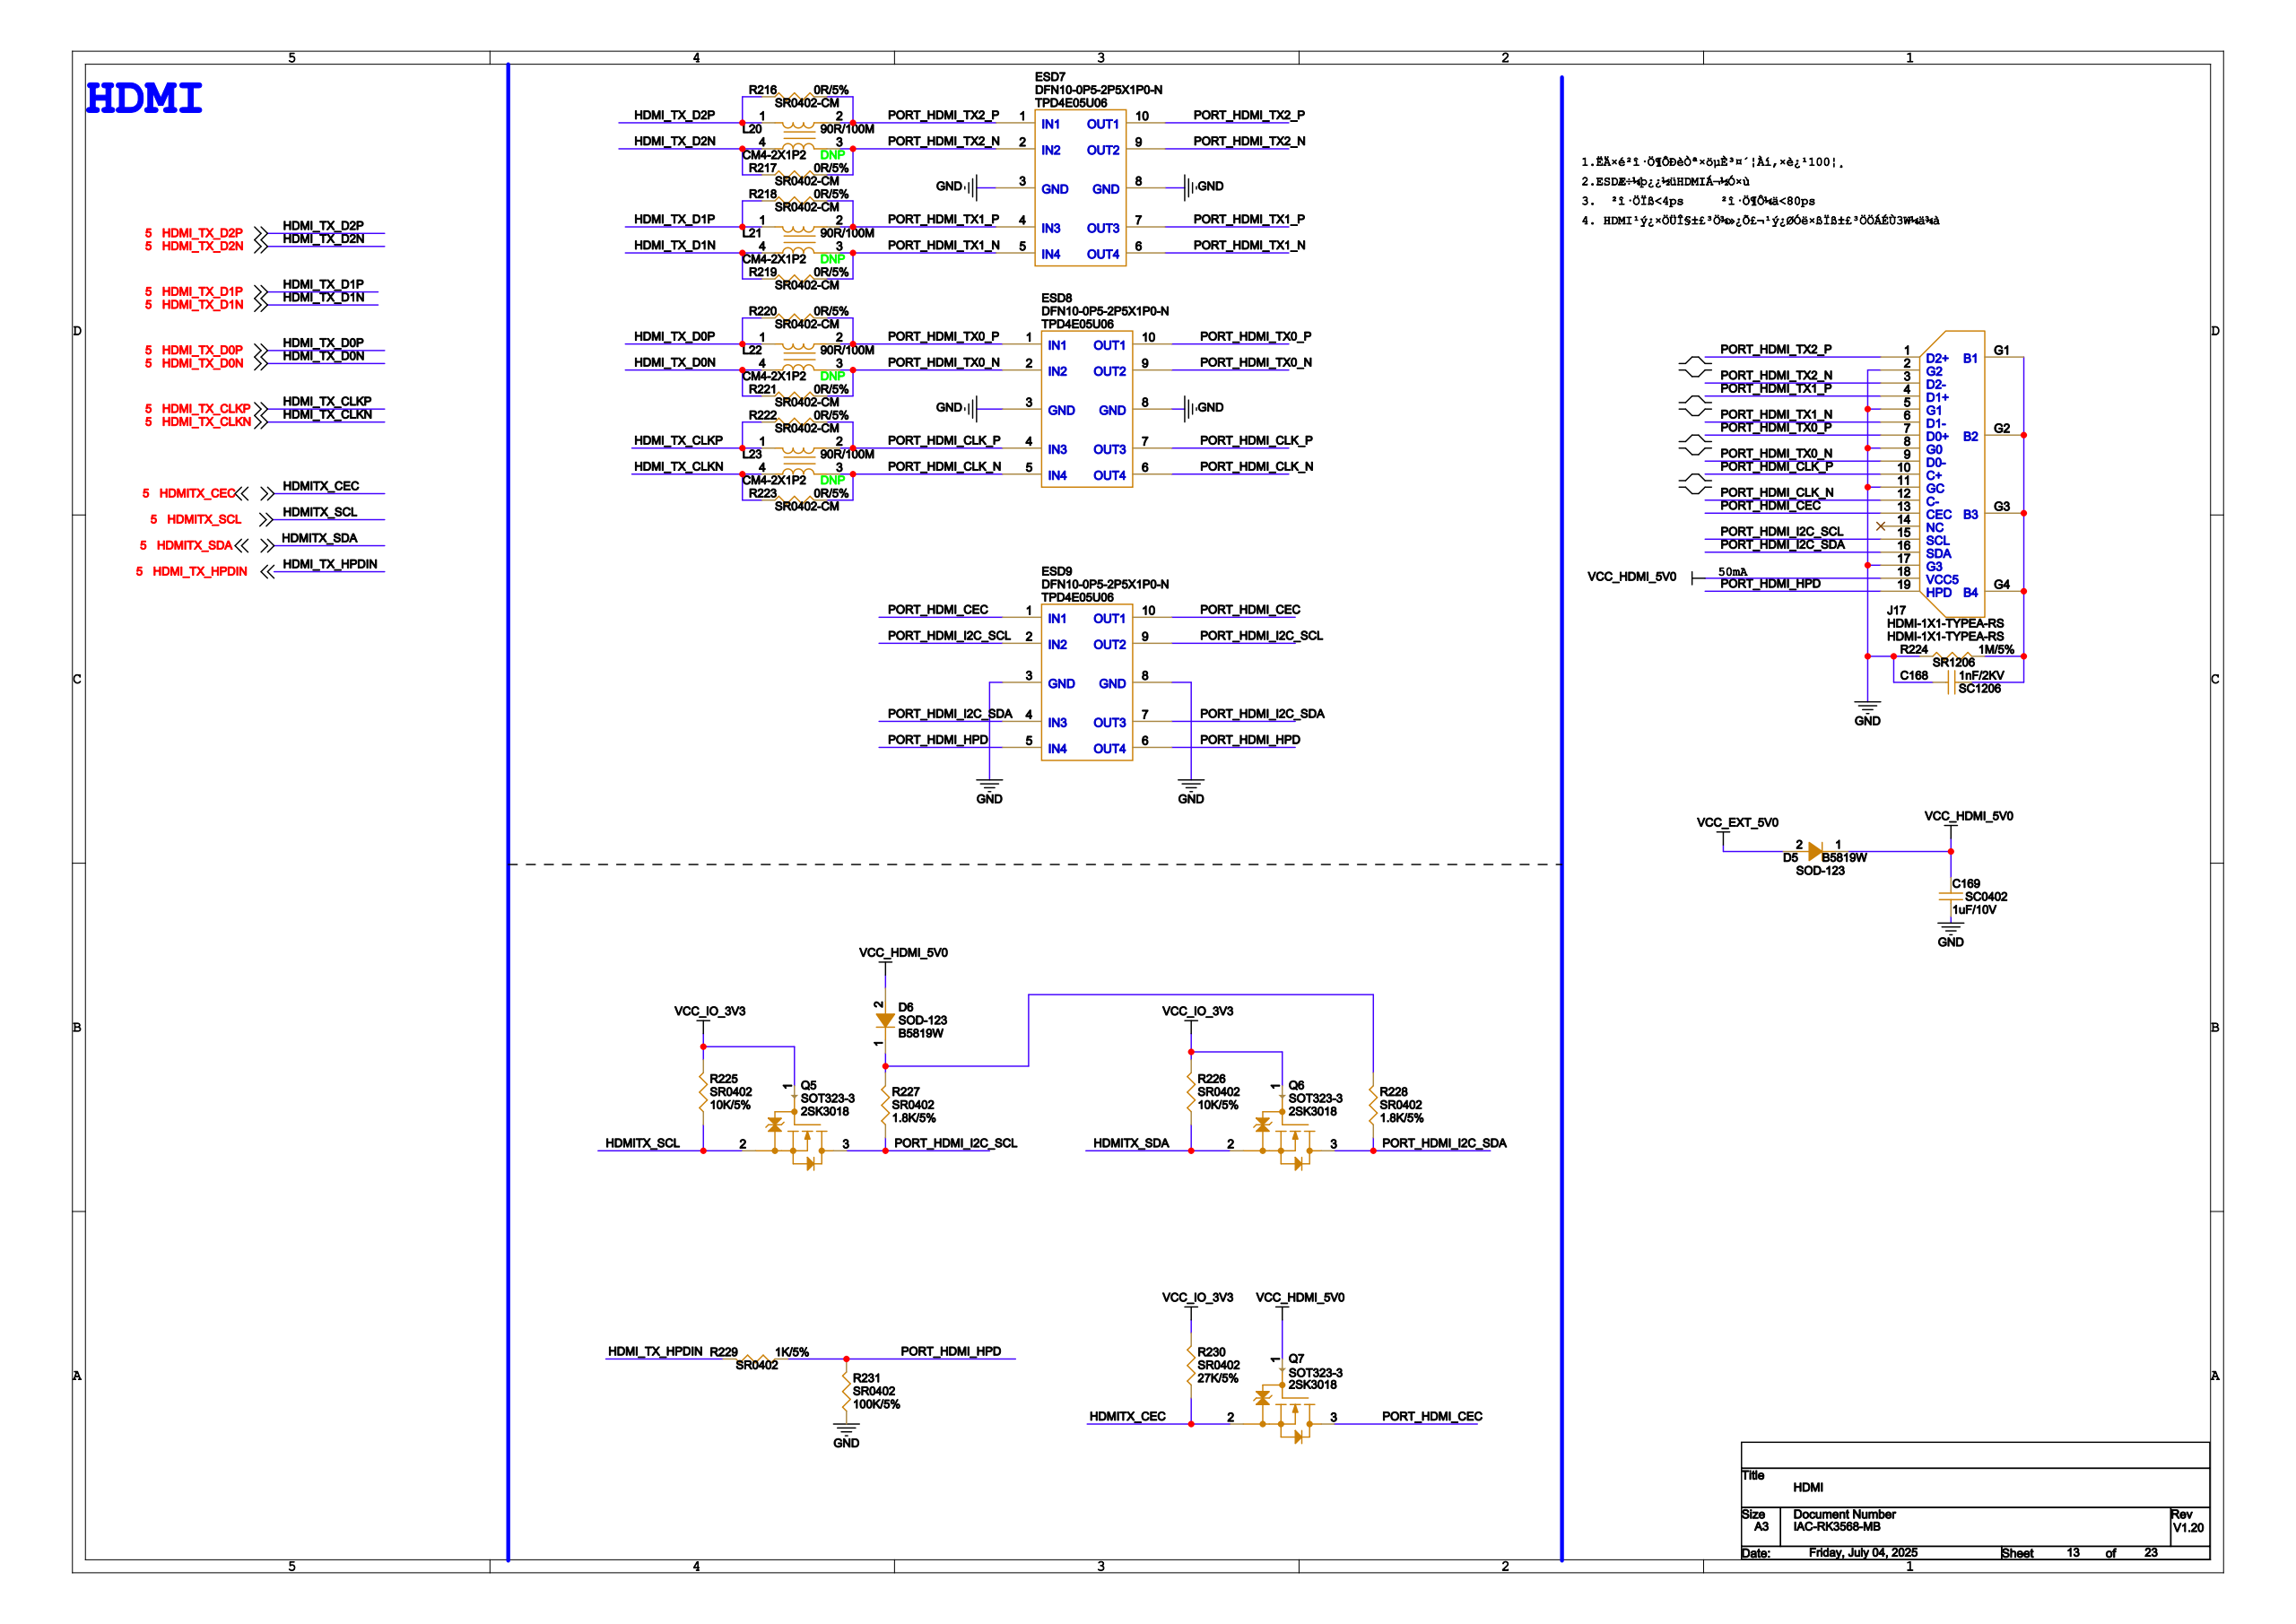Circuit board | Cadence Allegro | 1138 parts | 722 nets | one sheet of the schematic
Parts on this sheet (reference | value | footprint):
C168 | 1nF/2KV | SC1206
C169 | 1uF/10V | SC0402
D5 | B5819W | SOD-123
D6 | B5819W | SOD-123
ESD7 | TPD4E05U06 | DFN10-0P5-2P5X1P0-N
ESD8 | TPD4E05U06 | DFN10-0P5-2P5X1P0-N
ESD9 | TPD4E05U06 | DFN10-0P5-2P5X1P0-N
J17 | HDMI-1X1-TYPEA-RS | HDMI-1X1-TYPEA-RS
L20 | 90R/100M | CM4-2X1P2
L21 | 90R/100M | CM4-2X1P2
L22 | 90R/100M | CM4-2X1P2
L23 | 90R/100M | CM4-2X1P2
Q5 | 2SK3018 | SOT323-3
Q6 | 2SK3018 | SOT323-3
Q7 | 2SK3018 | SOT323-3
R216 | 0R/5% | SR0402-CM
R217 | 0R/5% | SR0402-CM
R218 | 0R/5% | SR0402-CM
R219 | 0R/5% | SR0402-CM
R220 | 0R/5% | SR0402-CM
R221 | 0R/5% | SR0402-CM
R222 | 0R/5% | SR0402-CM
R223 | 0R/5% | SR0402-CM
R224 | 1M/5% | SR1206
R225 | 10K/5% | SR0402
R226 | 10K/5% | SR0402
R227 | 1.8K/5% | SR0402
R228 | 1.8K/5% | SR0402
R229 | 1K/5% | SR0402
R230 | 27K/5% | SR0402
R231 | 100K/5% | SR0402
Nets of these parts (net: part-pin ...):
VCC_EXT_5V0: D5-2
VCC_HDMI_5V0: C169-1 D5-1 D6-2 Q7-1 J17-18
N4073020: D6-1 R227-2 R228-2
GND: C168-1 C169-2 ESD7-3 ESD7-8 ESD8-3 ESD8-8 ESD9-3 ESD9-8 R224-1 R231-1 J17-2 J17-5 J17-8 J17-11 J17-17
HDMI_TX_D2P: L20-1 R216-1
PORT_HDMI_TX2_P: ESD7-1 ESD7-10 L20-2 R216-2 J17-1
HDMI_TX_D2N: L20-4 R217-1
PORT_HDMI_TX2_N: ESD7-2 ESD7-9 L20-3 R217-2 J17-3
HDMI_TX_D1P: L21-1 R218-1
PORT_HDMI_TX1_P: ESD7-4 ESD7-7 L21-2 R218-2 J17-4
HDMI_TX_D1N: L21-4 R219-1
PORT_HDMI_TX1_N: ESD7-5 ESD7-6 L21-3 R219-2 J17-6
HDMI_TX_D0P: L22-1 R220-1
PORT_HDMI_TX0_P: ESD8-1 ESD8-10 L22-2 R220-2 J17-7
HDMI_TX_D0N: L22-4 R221-1
PORT_HDMI_TX0_N: ESD8-2 ESD8-9 L22-3 R221-2 J17-9
HDMI_TX_CLKP: L23-1 R222-1
PORT_HDMI_CLK_P: ESD8-4 ESD8-7 L23-2 R222-2 J17-10
HDMI_TX_CLKN: L23-4 R223-1
PORT_HDMI_CLK_N: ESD8-5 ESD8-6 L23-3 R223-2 J17-12
PORT_HDMI_I2C_SCL: ESD9-2 ESD9-9 Q5-3 R227-1 J17-15
HDMITX_SCL: Q5-2 R225-1
VCC_IO_3V3: Q5-1 Q6-1 R225-2 R226-2 R230-2
PORT_HDMI_I2C_SDA: ESD9-4 ESD9-7 Q6-3 R228-1 J17-16
HDMITX_SDA: Q6-2 R226-1
PORT_HDMI_CEC: ESD9-1 ESD9-10 Q7-3 J17-13
HDMITX_CEC: Q7-2 R230-1
N19507013: C168-2 R224-2 J17-G1 J17-G2 J17-G3 J17-G4
PORT_HDMI_HPD: ESD9-5 ESD9-6 R229-1 R231-2 J17-19
HDMI_TX_HPDIN: R229-2